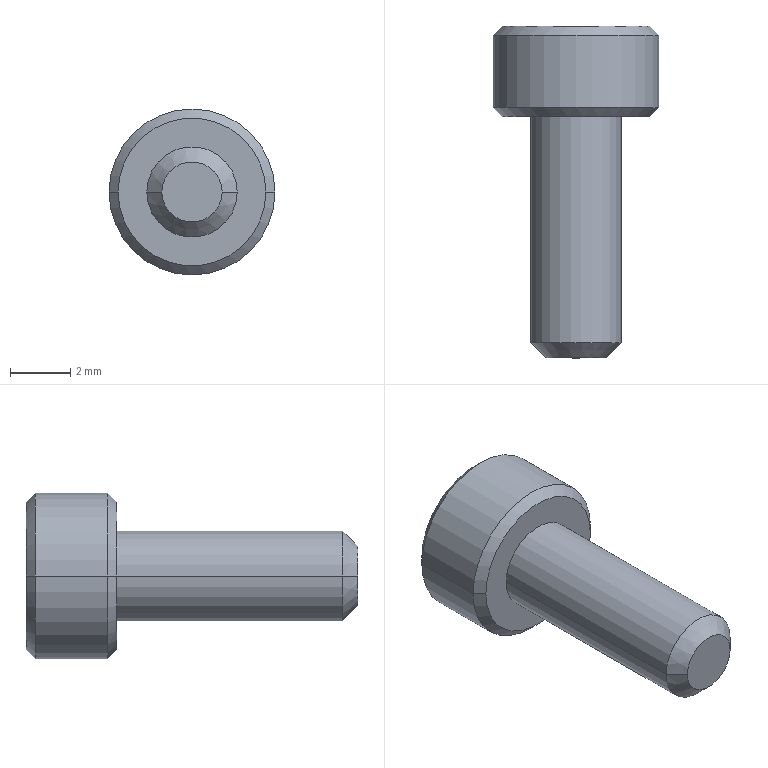Part | STEP file | BB62-M3-8L | 1 solid | 27 faces | box 5.5 x 11 x 5.5 mm | volume 116.536 mm3 | plane 15 | cone 8 | cylinder 4 | commonest cylinder face diameters 3 x2 5.5 x2
STEP:
#1=CARTESIAN_POINT('',(0.,0.8715,0.));
#2=VERTEX_POINT('',#1);
#3=CARTESIAN_POINT('',(1.435,1.7,0.));
#4=VERTEX_POINT('',#3);
#5=CARTESIAN_POINT('',(0.,0.8715,0.));
#6=DIRECTION('',(0.866,0.5,0.));
#7=VECTOR('',#6,1000.);
#8=LINE('',#5,#7);
#9=EDGE_CURVE('',#2,#4,#8,.T.);
#10=ORIENTED_EDGE('',*,*,#9,.F.);
#11=CARTESIAN_POINT('',(-1.435,1.7,0.));
#12=VERTEX_POINT('',#11);
#13=CARTESIAN_POINT('',(0.,0.8715,0.));
#14=DIRECTION('',(-0.866,0.5,0.));
#15=VECTOR('',#14,1000.);
#16=LINE('',#13,#15);
#17=EDGE_CURVE('',#2,#12,#16,.T.);
#18=ORIENTED_EDGE('',*,*,#17,.T.);
#19=CARTESIAN_POINT('',(-1.243,1.7,0.7175));
#20=VERTEX_POINT('',#19);
#21=CARTESIAN_POINT('',(0.,1.7,0.));
#22=DIRECTION('',(0.,-1.,0.));
#23=DIRECTION('',(-1.,0.,0.));
#24=AXIS2_PLACEMENT_3D('',#21,#22,#23);
#25=CIRCLE('',#24,1.435);
#26=EDGE_CURVE('',#20,#12,#25,.T.);
#27=ORIENTED_EDGE('',*,*,#26,.F.);
#28=CARTESIAN_POINT('',(0.,1.7,1.435));
#29=VERTEX_POINT('',#28);
#30=CARTESIAN_POINT('',(0.,1.7,0.));
#31=DIRECTION('',(0.,-1.,0.));
#32=DIRECTION('',(-1.,0.,0.));
#33=AXIS2_PLACEMENT_3D('',#30,#31,#32);
#34=CIRCLE('',#33,1.435);
#35=EDGE_CURVE('',#29,#20,#34,.T.);
#36=ORIENTED_EDGE('',*,*,#35,.F.);
#37=CARTESIAN_POINT('',(1.243,1.7,0.7175));
#38=VERTEX_POINT('',#37);
#39=CARTESIAN_POINT('',(0.,1.7,0.));
#40=DIRECTION('',(0.,-1.,0.));
#41=DIRECTION('',(-1.,0.,0.));
#42=AXIS2_PLACEMENT_3D('',#39,#40,#41);
#43=CIRCLE('',#42,1.435);
#44=EDGE_CURVE('',#38,#29,#43,.T.);
#45=ORIENTED_EDGE('',*,*,#44,.F.);
#46=CARTESIAN_POINT('',(0.,1.7,0.));
#47=DIRECTION('',(0.,-1.,0.));
#48=DIRECTION('',(-1.,0.,0.));
#49=AXIS2_PLACEMENT_3D('',#46,#47,#48);
#50=CIRCLE('',#49,1.435);
#51=EDGE_CURVE('',#4,#38,#50,.T.);
#52=ORIENTED_EDGE('',*,*,#51,.F.);
#53=EDGE_LOOP('',(#10,#18,#27,#36,#45,#52));
#54=FACE_OUTER_BOUND('',#53,.T.);
#55=CARTESIAN_POINT('',(0.,1000.872,0.));
#56=DIRECTION('',(0.,1.,0.));
#57=DIRECTION('',(1.,0.,0.));
#58=AXIS2_PLACEMENT_3D('',#55,#56,#57);
#59=CONICAL_SURFACE('',#58,1732.051,1.047);
#60=ADVANCED_FACE('',(#54),#59,.F.);
#61=CARTESIAN_POINT('',(1.,-8.,0.));
#62=VERTEX_POINT('',#61);
#63=CARTESIAN_POINT('',(-1.,-8.,0.));
#64=VERTEX_POINT('',#63);
#65=CARTESIAN_POINT('',(0.,-8.,0.));
#66=DIRECTION('',(0.,1.,0.));
#67=DIRECTION('',(1.,0.,0.));
#68=AXIS2_PLACEMENT_3D('',#65,#66,#67);
#69=CIRCLE('',#68,1.);
#70=EDGE_CURVE('',#62,#64,#69,.T.);
#71=ORIENTED_EDGE('',*,*,#70,.T.);
#72=CARTESIAN_POINT('',(-1.5,-7.5,0.));
#73=VERTEX_POINT('',#72);
#74=CARTESIAN_POINT('',(-1.,-8.,0.));
#75=DIRECTION('',(-0.7071,0.7071,0.));
#76=VECTOR('',#75,1000.);
#77=LINE('',#74,#76);
#78=EDGE_CURVE('',#64,#73,#77,.T.);
#79=ORIENTED_EDGE('',*,*,#78,.T.);
#80=CARTESIAN_POINT('',(1.5,-7.5,0.));
#81=VERTEX_POINT('',#80);
#82=CARTESIAN_POINT('',(0.,-7.5,0.));
#83=DIRECTION('',(0.,-1.,0.));
#84=DIRECTION('',(-1.,0.,0.));
#85=AXIS2_PLACEMENT_3D('',#82,#83,#84);
#86=CIRCLE('',#85,1.5);
#87=EDGE_CURVE('',#73,#81,#86,.T.);
#88=ORIENTED_EDGE('',*,*,#87,.T.);
#89=CARTESIAN_POINT('',(1.,-8.,0.));
#90=DIRECTION('',(0.7071,0.7071,0.));
#91=VECTOR('',#90,1000.);
#92=LINE('',#89,#91);
#93=EDGE_CURVE('',#62,#81,#92,.T.);
#94=ORIENTED_EDGE('',*,*,#93,.F.);
#95=EDGE_LOOP('',(#71,#79,#88,#94));
#96=FACE_OUTER_BOUND('',#95,.T.);
#97=CARTESIAN_POINT('',(0.,-8.,0.));
#98=DIRECTION('',(0.,1.,0.));
#99=DIRECTION('',(1.,0.,0.));
#100=AXIS2_PLACEMENT_3D('',#97,#98,#99);
#101=CONICAL_SURFACE('',#100,1.,0.7854);
#102=ADVANCED_FACE('',(#96),#101,.T.);
#103=ORIENTED_EDGE('',*,*,#87,.F.);
#104=CARTESIAN_POINT('',(-1.5,0.,0.));
#105=VERTEX_POINT('',#104);
#106=CARTESIAN_POINT('',(-1.5,-7.5,0.));
#107=DIRECTION('',(0.,1.,0.));
#108=VECTOR('',#107,1000.);
#109=LINE('',#106,#108);
#110=EDGE_CURVE('',#73,#105,#109,.T.);
#111=ORIENTED_EDGE('',*,*,#110,.T.);
#112=CARTESIAN_POINT('',(1.5,0.,0.));
#113=VERTEX_POINT('',#112);
#114=CARTESIAN_POINT('',(0.,0.,0.));
#115=DIRECTION('',(0.,-1.,0.));
#116=DIRECTION('',(-1.,0.,0.));
#117=AXIS2_PLACEMENT_3D('',#114,#115,#116);
#118=CIRCLE('',#117,1.5);
#119=EDGE_CURVE('',#105,#113,#118,.T.);
#120=ORIENTED_EDGE('',*,*,#119,.T.);
#121=CARTESIAN_POINT('',(1.5,-7.5,0.));
#122=DIRECTION('',(0.,1.,0.));
#123=VECTOR('',#122,1000.);
#124=LINE('',#121,#123);
#125=EDGE_CURVE('',#81,#113,#124,.T.);
#126=ORIENTED_EDGE('',*,*,#125,.F.);
#127=EDGE_LOOP('',(#103,#111,#120,#126));
#128=FACE_OUTER_BOUND('',#127,.T.);
#129=CARTESIAN_POINT('',(0.,-7.5,0.));
#130=DIRECTION('',(0.,1.,0.));
#131=DIRECTION('',(1.,0.,0.));
#132=AXIS2_PLACEMENT_3D('',#129,#130,#131);
#133=CYLINDRICAL_SURFACE('',#132,1.5);
#134=ADVANCED_FACE('',(#128),#133,.T.);
#135=CARTESIAN_POINT('',(-2.45,3.,0.));
#136=VERTEX_POINT('',#135);
#137=CARTESIAN_POINT('',(2.45,3.,0.));
#138=VERTEX_POINT('',#137);
#139=CARTESIAN_POINT('',(0.,3.,0.));
#140=DIRECTION('',(0.,-1.,0.));
#141=DIRECTION('',(-1.,0.,0.));
#142=AXIS2_PLACEMENT_3D('',#139,#140,#141);
#143=CIRCLE('',#142,2.45);
#144=EDGE_CURVE('',#136,#138,#143,.T.);
#145=ORIENTED_EDGE('',*,*,#144,.T.);
#146=CARTESIAN_POINT('',(2.75,2.7,0.));
#147=VERTEX_POINT('',#146);
#148=CARTESIAN_POINT('',(2.75,2.7,0.));
#149=DIRECTION('',(0.7071,-0.7071,0.));
#150=VECTOR('',#149,1000.);
#151=LINE('',#148,#150);
#152=EDGE_CURVE('',#138,#147,#151,.T.);
#153=ORIENTED_EDGE('',*,*,#152,.T.);
#154=CARTESIAN_POINT('',(-2.75,2.7,0.));
#155=VERTEX_POINT('',#154);
#156=CARTESIAN_POINT('',(0.,2.7,0.));
#157=DIRECTION('',(0.,-1.,0.));
#158=DIRECTION('',(-1.,0.,0.));
#159=AXIS2_PLACEMENT_3D('',#156,#157,#158);
#160=CIRCLE('',#159,2.75);
#161=EDGE_CURVE('',#155,#147,#160,.T.);
#162=ORIENTED_EDGE('',*,*,#161,.F.);
#163=CARTESIAN_POINT('',(-2.75,2.7,0.));
#164=DIRECTION('',(-0.7071,-0.7071,0.));
#165=VECTOR('',#164,1000.);
#166=LINE('',#163,#165);
#167=EDGE_CURVE('',#136,#155,#166,.T.);
#168=ORIENTED_EDGE('',*,*,#167,.F.);
#169=EDGE_LOOP('',(#145,#153,#162,#168));
#170=FACE_OUTER_BOUND('',#169,.T.);
#171=CARTESIAN_POINT('',(0.,2.7,0.));
#172=DIRECTION('',(0.,-1.,0.));
#173=DIRECTION('',(-1.,0.,0.));
#174=AXIS2_PLACEMENT_3D('',#171,#172,#173);
#175=CONICAL_SURFACE('',#174,2.75,0.7854);
#176=ADVANCED_FACE('',(#170),#175,.T.);
#177=ORIENTED_EDGE('',*,*,#161,.T.);
#178=CARTESIAN_POINT('',(2.75,0.3,0.));
#179=VERTEX_POINT('',#178);
#180=CARTESIAN_POINT('',(2.75,1.62,0.));
#181=DIRECTION('',(0.,-1.,0.));
#182=VECTOR('',#181,1000.);
#183=LINE('',#180,#182);
#184=EDGE_CURVE('',#147,#179,#183,.T.);
#185=ORIENTED_EDGE('',*,*,#184,.T.);
#186=CARTESIAN_POINT('',(-2.75,0.3,0.));
#187=VERTEX_POINT('',#186);
#188=CARTESIAN_POINT('',(0.,0.3,0.));
#189=DIRECTION('',(0.,-1.,0.));
#190=DIRECTION('',(-1.,0.,0.));
#191=AXIS2_PLACEMENT_3D('',#188,#189,#190);
#192=CIRCLE('',#191,2.75);
#193=EDGE_CURVE('',#187,#179,#192,.T.);
#194=ORIENTED_EDGE('',*,*,#193,.F.);
#195=CARTESIAN_POINT('',(-2.75,1.62,0.));
#196=DIRECTION('',(0.,-1.,0.));
#197=VECTOR('',#196,1000.);
#198=LINE('',#195,#197);
#199=EDGE_CURVE('',#155,#187,#198,.T.);
#200=ORIENTED_EDGE('',*,*,#199,.F.);
#201=EDGE_LOOP('',(#177,#185,#194,#200));
#202=FACE_OUTER_BOUND('',#201,.T.);
#203=CARTESIAN_POINT('',(0.,1.62,0.));
#204=DIRECTION('',(0.,-1.,0.));
#205=DIRECTION('',(-1.,0.,0.));
#206=AXIS2_PLACEMENT_3D('',#203,#204,#205);
#207=CYLINDRICAL_SURFACE('',#206,2.75);
#208=ADVANCED_FACE('',(#202),#207,.T.);
#209=CARTESIAN_POINT('',(-2.45,0.,0.));
#210=VERTEX_POINT('',#209);
#211=CARTESIAN_POINT('',(2.45,0.,0.));
#212=VERTEX_POINT('',#211);
#213=CARTESIAN_POINT('',(0.,0.,0.));
#214=DIRECTION('',(0.,-1.,0.));
#215=DIRECTION('',(-1.,0.,0.));
#216=AXIS2_PLACEMENT_3D('',#213,#214,#215);
#217=CIRCLE('',#216,2.45);
#218=EDGE_CURVE('',#210,#212,#217,.T.);
#219=ORIENTED_EDGE('',*,*,#218,.F.);
#220=CARTESIAN_POINT('',(-2.45,0.,0.));
#221=DIRECTION('',(-0.7071,0.7071,0.));
#222=VECTOR('',#221,1000.);
#223=LINE('',#220,#222);
#224=EDGE_CURVE('',#210,#187,#223,.T.);
#225=ORIENTED_EDGE('',*,*,#224,.T.);
#226=ORIENTED_EDGE('',*,*,#193,.T.);
#227=CARTESIAN_POINT('',(2.45,0.,0.));
#228=DIRECTION('',(0.7071,0.7071,0.));
#229=VECTOR('',#228,1000.);
#230=LINE('',#227,#229);
#231=EDGE_CURVE('',#212,#179,#230,.T.);
#232=ORIENTED_EDGE('',*,*,#231,.F.);
#233=EDGE_LOOP('',(#219,#225,#226,#232));
#234=FACE_OUTER_BOUND('',#233,.T.);
#235=CARTESIAN_POINT('',(0.,0.,0.));
#236=DIRECTION('',(0.,1.,0.));
#237=DIRECTION('',(1.,0.,0.));
#238=AXIS2_PLACEMENT_3D('',#235,#236,#237);
#239=CONICAL_SURFACE('',#238,2.45,0.7854);
#240=ADVANCED_FACE('',(#234),#239,.T.);
#241=ORIENTED_EDGE('',*,*,#144,.F.);
#242=CARTESIAN_POINT('',(0.,3.,0.));
#243=DIRECTION('',(0.,-1.,0.));
#244=DIRECTION('',(-1.,0.,0.));
#245=AXIS2_PLACEMENT_3D('',#242,#243,#244);
#246=CIRCLE('',#245,2.45);
#247=EDGE_CURVE('',#138,#136,#246,.T.);
#248=ORIENTED_EDGE('',*,*,#247,.F.);
#249=EDGE_LOOP('',(#241,#248));
#250=FACE_OUTER_BOUND('',#249,.T.);
#251=CARTESIAN_POINT('',(0.,3.,-1.435));
#252=VERTEX_POINT('',#251);
#253=CARTESIAN_POINT('',(-1.243,3.,-0.7175));
#254=VERTEX_POINT('',#253);
#255=CARTESIAN_POINT('',(0.,3.,-1.435));
#256=DIRECTION('',(-0.866,0.,0.5));
#257=VECTOR('',#256,1000.);
#258=LINE('',#255,#257);
#259=EDGE_CURVE('',#252,#254,#258,.T.);
#260=ORIENTED_EDGE('',*,*,#259,.F.);
#261=CARTESIAN_POINT('',(1.243,3.,-0.7175));
#262=VERTEX_POINT('',#261);
#263=CARTESIAN_POINT('',(1.243,3.,-0.7175));
#264=DIRECTION('',(-0.866,0.,-0.5));
#265=VECTOR('',#264,1000.);
#266=LINE('',#263,#265);
#267=EDGE_CURVE('',#262,#252,#266,.T.);
#268=ORIENTED_EDGE('',*,*,#267,.F.);
#269=CARTESIAN_POINT('',(1.243,3.,0.7175));
#270=VERTEX_POINT('',#269);
#271=CARTESIAN_POINT('',(1.243,3.,0.7175));
#272=DIRECTION('',(0.,0.,-1.));
#273=VECTOR('',#272,1000.);
#274=LINE('',#271,#273);
#275=EDGE_CURVE('',#270,#262,#274,.T.);
#276=ORIENTED_EDGE('',*,*,#275,.F.);
#277=CARTESIAN_POINT('',(0.,3.,1.435));
#278=VERTEX_POINT('',#277);
#279=CARTESIAN_POINT('',(0.,3.,1.435));
#280=DIRECTION('',(0.866,0.,-0.5));
#281=VECTOR('',#280,1000.);
#282=LINE('',#279,#281);
#283=EDGE_CURVE('',#278,#270,#282,.T.);
#284=ORIENTED_EDGE('',*,*,#283,.F.);
#285=CARTESIAN_POINT('',(-1.243,3.,0.7175));
#286=VERTEX_POINT('',#285);
#287=CARTESIAN_POINT('',(-1.243,3.,0.7175));
#288=DIRECTION('',(0.866,0.,0.5));
#289=VECTOR('',#288,1000.);
#290=LINE('',#287,#289);
#291=EDGE_CURVE('',#286,#278,#290,.T.);
#292=ORIENTED_EDGE('',*,*,#291,.F.);
#293=CARTESIAN_POINT('',(-1.243,3.,-0.7175));
#294=DIRECTION('',(0.,0.,1.));
#295=VECTOR('',#294,1000.);
#296=LINE('',#293,#295);
#297=EDGE_CURVE('',#254,#286,#296,.T.);
#298=ORIENTED_EDGE('',*,*,#297,.F.);
#299=EDGE_LOOP('',(#260,#268,#276,#284,#292,#298));
#300=FACE_BOUND('',#299,.T.);
#301=CARTESIAN_POINT('',(2.45,3.,0.));
#302=DIRECTION('',(0.,1.,0.));
#303=DIRECTION('',(1.,0.,0.));
#304=AXIS2_PLACEMENT_3D('',#301,#302,#303);
#305=PLANE('',#304);
#306=ADVANCED_FACE('',(#250,#300),#305,.T.);
#307=CARTESIAN_POINT('',(0.,0.,0.));
#308=DIRECTION('',(0.,-1.,0.));
#309=DIRECTION('',(-1.,0.,0.));
#310=AXIS2_PLACEMENT_3D('',#307,#308,#309);
#311=CIRCLE('',#310,1.5);
#312=EDGE_CURVE('',#113,#105,#311,.T.);
#313=ORIENTED_EDGE('',*,*,#312,.F.);
#314=ORIENTED_EDGE('',*,*,#119,.F.);
#315=EDGE_LOOP('',(#313,#314));
#316=FACE_BOUND('',#315,.T.);
#317=CARTESIAN_POINT('',(0.,0.,0.));
#318=DIRECTION('',(0.,-1.,0.));
#319=DIRECTION('',(-1.,0.,0.));
#320=AXIS2_PLACEMENT_3D('',#317,#318,#319);
#321=CIRCLE('',#320,2.45);
#322=EDGE_CURVE('',#212,#210,#321,.T.);
#323=ORIENTED_EDGE('',*,*,#322,.T.);
#324=ORIENTED_EDGE('',*,*,#218,.T.);
#325=EDGE_LOOP('',(#323,#324));
#326=FACE_OUTER_BOUND('',#325,.T.);
#327=CARTESIAN_POINT('',(0.,0.,0.));
#328=DIRECTION('',(0.,-1.,0.));
#329=DIRECTION('',(-1.,0.,0.));
#330=AXIS2_PLACEMENT_3D('',#327,#328,#329);
#331=PLANE('',#330);
#332=ADVANCED_FACE('',(#316,#326),#331,.T.);
#333=ORIENTED_EDGE('',*,*,#224,.F.);
#334=ORIENTED_EDGE('',*,*,#322,.F.);
#335=ORIENTED_EDGE('',*,*,#231,.T.);
#336=CARTESIAN_POINT('',(0.,0.3,0.));
#337=DIRECTION('',(0.,-1.,0.));
#338=DIRECTION('',(-1.,0.,0.));
#339=AXIS2_PLACEMENT_3D('',#336,#337,#338);
#340=CIRCLE('',#339,2.75);
#341=EDGE_CURVE('',#179,#187,#340,.T.);
#342=ORIENTED_EDGE('',*,*,#341,.T.);
#343=EDGE_LOOP('',(#333,#334,#335,#342));
#344=FACE_OUTER_BOUND('',#343,.T.);
#345=CARTESIAN_POINT('',(0.,0.,0.));
#346=DIRECTION('',(0.,1.,0.));
#347=DIRECTION('',(1.,0.,0.));
#348=AXIS2_PLACEMENT_3D('',#345,#346,#347);
#349=CONICAL_SURFACE('',#348,2.45,0.7854);
#350=ADVANCED_FACE('',(#344),#349,.T.);
#351=ORIENTED_EDGE('',*,*,#184,.F.);
#352=CARTESIAN_POINT('',(0.,2.7,0.));
#353=DIRECTION('',(0.,-1.,0.));
#354=DIRECTION('',(-1.,0.,0.));
#355=AXIS2_PLACEMENT_3D('',#352,#353,#354);
#356=CIRCLE('',#355,2.75);
#357=EDGE_CURVE('',#147,#155,#356,.T.);
#358=ORIENTED_EDGE('',*,*,#357,.T.);
#359=ORIENTED_EDGE('',*,*,#199,.T.);
#360=ORIENTED_EDGE('',*,*,#341,.F.);
#361=EDGE_LOOP('',(#351,#358,#359,#360));
#362=FACE_OUTER_BOUND('',#361,.T.);
#363=CARTESIAN_POINT('',(0.,1.62,0.));
#364=DIRECTION('',(0.,-1.,0.));
#365=DIRECTION('',(-1.,0.,0.));
#366=AXIS2_PLACEMENT_3D('',#363,#364,#365);
#367=CYLINDRICAL_SURFACE('',#366,2.75);
#368=ADVANCED_FACE('',(#362),#367,.T.);
#369=ORIENTED_EDGE('',*,*,#152,.F.);
#370=ORIENTED_EDGE('',*,*,#247,.T.);
#371=ORIENTED_EDGE('',*,*,#167,.T.);
#372=ORIENTED_EDGE('',*,*,#357,.F.);
#373=EDGE_LOOP('',(#369,#370,#371,#372));
#374=FACE_OUTER_BOUND('',#373,.T.);
#375=CARTESIAN_POINT('',(0.,2.7,0.));
#376=DIRECTION('',(0.,-1.,0.));
#377=DIRECTION('',(-1.,0.,0.));
#378=AXIS2_PLACEMENT_3D('',#375,#376,#377);
#379=CONICAL_SURFACE('',#378,2.75,0.7854);
#380=ADVANCED_FACE('',(#374),#379,.T.);
#381=ORIENTED_EDGE('',*,*,#110,.F.);
#382=CARTESIAN_POINT('',(0.,-7.5,0.));
#383=DIRECTION('',(0.,-1.,0.));
#384=DIRECTION('',(-1.,0.,0.));
#385=AXIS2_PLACEMENT_3D('',#382,#383,#384);
#386=CIRCLE('',#385,1.5);
#387=EDGE_CURVE('',#81,#73,#386,.T.);
#388=ORIENTED_EDGE('',*,*,#387,.F.);
#389=ORIENTED_EDGE('',*,*,#125,.T.);
#390=ORIENTED_EDGE('',*,*,#312,.T.);
#391=EDGE_LOOP('',(#381,#388,#389,#390));
#392=FACE_OUTER_BOUND('',#391,.T.);
#393=CARTESIAN_POINT('',(0.,-7.5,0.));
#394=DIRECTION('',(0.,1.,0.));
#395=DIRECTION('',(1.,0.,0.));
#396=AXIS2_PLACEMENT_3D('',#393,#394,#395);
#397=CYLINDRICAL_SURFACE('',#396,1.5);
#398=ADVANCED_FACE('',(#392),#397,.T.);
#399=ORIENTED_EDGE('',*,*,#70,.F.);
#400=CARTESIAN_POINT('',(0.,-8.,0.));
#401=DIRECTION('',(0.,1.,0.));
#402=DIRECTION('',(1.,0.,0.));
#403=AXIS2_PLACEMENT_3D('',#400,#401,#402);
#404=CIRCLE('',#403,1.);
#405=EDGE_CURVE('',#64,#62,#404,.T.);
#406=ORIENTED_EDGE('',*,*,#405,.F.);
#407=EDGE_LOOP('',(#399,#406));
#408=FACE_OUTER_BOUND('',#407,.T.);
#409=CARTESIAN_POINT('',(0.,-8.,0.));
#410=DIRECTION('',(0.,-1.,0.));
#411=DIRECTION('',(-1.,0.,0.));
#412=AXIS2_PLACEMENT_3D('',#409,#410,#411);
#413=PLANE('',#412);
#414=ADVANCED_FACE('',(#408),#413,.T.);
#415=ORIENTED_EDGE('',*,*,#78,.F.);
#416=ORIENTED_EDGE('',*,*,#405,.T.);
#417=ORIENTED_EDGE('',*,*,#93,.T.);
#418=ORIENTED_EDGE('',*,*,#387,.T.);
#419=EDGE_LOOP('',(#415,#416,#417,#418));
#420=FACE_OUTER_BOUND('',#419,.T.);
#421=CARTESIAN_POINT('',(0.,-8.,0.));
#422=DIRECTION('',(0.,1.,0.));
#423=DIRECTION('',(1.,0.,0.));
#424=AXIS2_PLACEMENT_3D('',#421,#422,#423);
#425=CONICAL_SURFACE('',#424,1.,0.7854);
#426=ADVANCED_FACE('',(#420),#425,.T.);
#427=CARTESIAN_POINT('',(1.243,1.7,-0.7175));
#428=VERTEX_POINT('',#427);
#429=CARTESIAN_POINT('',(0.,1.7,-1.435));
#430=VERTEX_POINT('',#429);
#431=CARTESIAN_POINT('',(1.243,1.7,-0.7175));
#432=DIRECTION('',(-0.866,0.,-0.5));
#433=VECTOR('',#432,1000.);
#434=LINE('',#431,#433);
#435=EDGE_CURVE('',#428,#430,#434,.T.);
#436=ORIENTED_EDGE('',*,*,#435,.F.);
#437=CARTESIAN_POINT('',(1.243,3.,-0.7175));
#438=DIRECTION('',(0.,-1.,0.));
#439=VECTOR('',#438,1000.);
#440=LINE('',#437,#439);
#441=EDGE_CURVE('',#262,#428,#440,.T.);
#442=ORIENTED_EDGE('',*,*,#441,.F.);
#443=ORIENTED_EDGE('',*,*,#267,.T.);
#444=CARTESIAN_POINT('',(0.,3.,-1.435));
#445=DIRECTION('',(0.,-1.,0.));
#446=VECTOR('',#445,1000.);
#447=LINE('',#444,#446);
#448=EDGE_CURVE('',#252,#430,#447,.T.);
#449=ORIENTED_EDGE('',*,*,#448,.T.);
#450=EDGE_LOOP('',(#436,#442,#443,#449));
#451=FACE_OUTER_BOUND('',#450,.T.);
#452=CARTESIAN_POINT('',(1.243,3.,-0.7175));
#453=DIRECTION('',(-0.5,0.,0.866));
#454=DIRECTION('',(0.866,0.,0.5));
#455=AXIS2_PLACEMENT_3D('',#452,#453,#454);
#456=PLANE('',#455);
#457=ADVANCED_FACE('',(#451),#456,.T.);
#458=CARTESIAN_POINT('',(-1.243,1.7,-0.7175));
#459=VERTEX_POINT('',#458);
#460=CARTESIAN_POINT('',(0.,1.7,-1.435));
#461=DIRECTION('',(-0.866,0.,0.5));
#462=VECTOR('',#461,1000.);
#463=LINE('',#460,#462);
#464=EDGE_CURVE('',#430,#459,#463,.T.);
#465=ORIENTED_EDGE('',*,*,#464,.F.);
#466=ORIENTED_EDGE('',*,*,#448,.F.);
#467=ORIENTED_EDGE('',*,*,#259,.T.);
#468=CARTESIAN_POINT('',(-1.243,3.,-0.7175));
#469=DIRECTION('',(0.,-1.,0.));
#470=VECTOR('',#469,1000.);
#471=LINE('',#468,#470);
#472=EDGE_CURVE('',#254,#459,#471,.T.);
#473=ORIENTED_EDGE('',*,*,#472,.T.);
#474=EDGE_LOOP('',(#465,#466,#467,#473));
#475=FACE_OUTER_BOUND('',#474,.T.);
#476=CARTESIAN_POINT('',(0.,3.,-1.435));
#477=DIRECTION('',(0.5,0.,0.866));
#478=DIRECTION('',(0.866,0.,-0.5));
#479=AXIS2_PLACEMENT_3D('',#476,#477,#478);
#480=PLANE('',#479);
#481=ADVANCED_FACE('',(#475),#480,.T.);
#482=CARTESIAN_POINT('',(-1.243,1.7,-0.7175));
#483=DIRECTION('',(0.,0.,1.));
#484=VECTOR('',#483,1000.);
#485=LINE('',#482,#484);
#486=EDGE_CURVE('',#459,#20,#485,.T.);
#487=ORIENTED_EDGE('',*,*,#486,.F.);
#488=ORIENTED_EDGE('',*,*,#472,.F.);
#489=ORIENTED_EDGE('',*,*,#297,.T.);
#490=CARTESIAN_POINT('',(-1.243,3.,0.7175));
#491=DIRECTION('',(0.,-1.,0.));
#492=VECTOR('',#491,1000.);
#493=LINE('',#490,#492);
#494=EDGE_CURVE('',#286,#20,#493,.T.);
#495=ORIENTED_EDGE('',*,*,#494,.T.);
#496=EDGE_LOOP('',(#487,#488,#489,#495));
#497=FACE_OUTER_BOUND('',#496,.T.);
#498=CARTESIAN_POINT('',(-1.243,3.,-0.7175));
#499=DIRECTION('',(1.,0.,0.));
#500=DIRECTION('',(0.,0.,-1.));
#501=AXIS2_PLACEMENT_3D('',#498,#499,#500);
#502=PLANE('',#501);
#503=ADVANCED_FACE('',(#497),#502,.T.);
#504=CARTESIAN_POINT('',(-1.243,1.7,0.7175));
#505=DIRECTION('',(0.866,0.,0.5));
#506=VECTOR('',#505,1000.);
#507=LINE('',#504,#506);
#508=EDGE_CURVE('',#20,#29,#507,.T.);
#509=ORIENTED_EDGE('',*,*,#508,.F.);
#510=ORIENTED_EDGE('',*,*,#494,.F.);
#511=ORIENTED_EDGE('',*,*,#291,.T.);
#512=CARTESIAN_POINT('',(0.,3.,1.435));
#513=DIRECTION('',(0.,-1.,0.));
#514=VECTOR('',#513,1000.);
#515=LINE('',#512,#514);
#516=EDGE_CURVE('',#278,#29,#515,.T.);
#517=ORIENTED_EDGE('',*,*,#516,.T.);
#518=EDGE_LOOP('',(#509,#510,#511,#517));
#519=FACE_OUTER_BOUND('',#518,.T.);
#520=CARTESIAN_POINT('',(-1.243,3.,0.7175));
#521=DIRECTION('',(0.5,0.,-0.866));
#522=DIRECTION('',(-0.866,0.,-0.5));
#523=AXIS2_PLACEMENT_3D('',#520,#521,#522);
#524=PLANE('',#523);
#525=ADVANCED_FACE('',(#519),#524,.T.);
#526=CARTESIAN_POINT('',(0.,1.7,1.435));
#527=DIRECTION('',(0.866,0.,-0.5));
#528=VECTOR('',#527,1000.);
#529=LINE('',#526,#528);
#530=EDGE_CURVE('',#29,#38,#529,.T.);
#531=ORIENTED_EDGE('',*,*,#530,.F.);
#532=ORIENTED_EDGE('',*,*,#516,.F.);
#533=ORIENTED_EDGE('',*,*,#283,.T.);
#534=CARTESIAN_POINT('',(1.243,3.,0.7175));
#535=DIRECTION('',(0.,-1.,0.));
#536=VECTOR('',#535,1000.);
#537=LINE('',#534,#536);
#538=EDGE_CURVE('',#270,#38,#537,.T.);
#539=ORIENTED_EDGE('',*,*,#538,.T.);
#540=EDGE_LOOP('',(#531,#532,#533,#539));
#541=FACE_OUTER_BOUND('',#540,.T.);
#542=CARTESIAN_POINT('',(0.,3.,1.435));
#543=DIRECTION('',(-0.5,0.,-0.866));
#544=DIRECTION('',(-0.866,0.,0.5));
#545=AXIS2_PLACEMENT_3D('',#542,#543,#544);
#546=PLANE('',#545);
#547=ADVANCED_FACE('',(#541),#546,.T.);
#548=CARTESIAN_POINT('',(1.243,1.7,0.7175));
#549=DIRECTION('',(0.,0.,-1.));
#550=VECTOR('',#549,1000.);
#551=LINE('',#548,#550);
#552=EDGE_CURVE('',#38,#428,#551,.T.);
#553=ORIENTED_EDGE('',*,*,#552,.F.);
#554=ORIENTED_EDGE('',*,*,#538,.F.);
#555=ORIENTED_EDGE('',*,*,#275,.T.);
#556=ORIENTED_EDGE('',*,*,#441,.T.);
#557=EDGE_LOOP('',(#553,#554,#555,#556));
#558=FACE_OUTER_BOUND('',#557,.T.);
#559=CARTESIAN_POINT('',(1.243,3.,0.7175));
#560=DIRECTION('',(-1.,0.,0.));
#561=DIRECTION('',(0.,0.,1.));
#562=AXIS2_PLACEMENT_3D('',#559,#560,#561);
#563=PLANE('',#562);
#564=ADVANCED_FACE('',(#558),#563,.T.);
#565=ORIENTED_EDGE('',*,*,#435,.T.);
#566=CARTESIAN_POINT('',(0.,1.7,0.));
#567=DIRECTION('',(0.,-1.,0.));
#568=DIRECTION('',(-1.,0.,0.));
#569=AXIS2_PLACEMENT_3D('',#566,#567,#568);
#570=CIRCLE('',#569,1.435);
#571=EDGE_CURVE('',#430,#428,#570,.T.);
#572=ORIENTED_EDGE('',*,*,#571,.T.);
#573=EDGE_LOOP('',(#565,#572));
#574=FACE_OUTER_BOUND('',#573,.T.);
#575=CARTESIAN_POINT('',(0.,1.7,0.));
#576=DIRECTION('',(0.,1.,0.));
#577=DIRECTION('',(1.,0.,0.));
#578=AXIS2_PLACEMENT_3D('',#575,#576,#577);
#579=PLANE('',#578);
#580=ADVANCED_FACE('',(#574),#579,.F.);
#581=ORIENTED_EDGE('',*,*,#552,.T.);
#582=CARTESIAN_POINT('',(0.,1.7,0.));
#583=DIRECTION('',(0.,-1.,0.));
#584=DIRECTION('',(-1.,0.,0.));
#585=AXIS2_PLACEMENT_3D('',#582,#583,#584);
#586=CIRCLE('',#585,1.435);
#587=EDGE_CURVE('',#428,#4,#586,.T.);
#588=ORIENTED_EDGE('',*,*,#587,.T.);
#589=ORIENTED_EDGE('',*,*,#51,.T.);
#590=EDGE_LOOP('',(#581,#588,#589));
#591=FACE_OUTER_BOUND('',#590,.T.);
#592=CARTESIAN_POINT('',(0.,1.7,0.));
#593=DIRECTION('',(0.,1.,0.));
#594=DIRECTION('',(1.,0.,0.));
#595=AXIS2_PLACEMENT_3D('',#592,#593,#594);
#596=PLANE('',#595);
#597=ADVANCED_FACE('',(#591),#596,.F.);
#598=ORIENTED_EDGE('',*,*,#530,.T.);
#599=ORIENTED_EDGE('',*,*,#44,.T.);
#600=EDGE_LOOP('',(#598,#599));
#601=FACE_OUTER_BOUND('',#600,.T.);
#602=CARTESIAN_POINT('',(0.,1.7,0.));
#603=DIRECTION('',(0.,1.,0.));
#604=DIRECTION('',(1.,0.,0.));
#605=AXIS2_PLACEMENT_3D('',#602,#603,#604);
#606=PLANE('',#605);
#607=ADVANCED_FACE('',(#601),#606,.F.);
#608=ORIENTED_EDGE('',*,*,#508,.T.);
#609=ORIENTED_EDGE('',*,*,#35,.T.);
#610=EDGE_LOOP('',(#608,#609));
#611=FACE_OUTER_BOUND('',#610,.T.);
#612=CARTESIAN_POINT('',(0.,1.7,0.));
#613=DIRECTION('',(0.,1.,0.));
#614=DIRECTION('',(1.,0.,0.));
#615=AXIS2_PLACEMENT_3D('',#612,#613,#614);
#616=PLANE('',#615);
#617=ADVANCED_FACE('',(#611),#616,.F.);
#618=ORIENTED_EDGE('',*,*,#486,.T.);
#619=ORIENTED_EDGE('',*,*,#26,.T.);
#620=CARTESIAN_POINT('',(0.,1.7,0.));
#621=DIRECTION('',(0.,-1.,0.));
#622=DIRECTION('',(-1.,0.,0.));
#623=AXIS2_PLACEMENT_3D('',#620,#621,#622);
#624=CIRCLE('',#623,1.435);
#625=EDGE_CURVE('',#12,#459,#624,.T.);
#626=ORIENTED_EDGE('',*,*,#625,.T.);
#627=EDGE_LOOP('',(#618,#619,#626));
#628=FACE_OUTER_BOUND('',#627,.T.);
#629=CARTESIAN_POINT('',(0.,1.7,0.));
#630=DIRECTION('',(0.,1.,0.));
#631=DIRECTION('',(1.,0.,0.));
#632=AXIS2_PLACEMENT_3D('',#629,#630,#631);
#633=PLANE('',#632);
#634=ADVANCED_FACE('',(#628),#633,.F.);
#635=ORIENTED_EDGE('',*,*,#464,.T.);
#636=CARTESIAN_POINT('',(0.,1.7,0.));
#637=DIRECTION('',(0.,-1.,0.));
#638=DIRECTION('',(-1.,0.,0.));
#639=AXIS2_PLACEMENT_3D('',#636,#637,#638);
#640=CIRCLE('',#639,1.435);
#641=EDGE_CURVE('',#459,#430,#640,.T.);
#642=ORIENTED_EDGE('',*,*,#641,.T.);
#643=EDGE_LOOP('',(#635,#642));
#644=FACE_OUTER_BOUND('',#643,.T.);
#645=CARTESIAN_POINT('',(0.,1.7,0.));
#646=DIRECTION('',(0.,1.,0.));
#647=DIRECTION('',(1.,0.,0.));
#648=AXIS2_PLACEMENT_3D('',#645,#646,#647);
#649=PLANE('',#648);
#650=ADVANCED_FACE('',(#644),#649,.F.);
#651=ORIENTED_EDGE('',*,*,#17,.F.);
#652=ORIENTED_EDGE('',*,*,#9,.T.);
#653=ORIENTED_EDGE('',*,*,#587,.F.);
#654=ORIENTED_EDGE('',*,*,#571,.F.);
#655=ORIENTED_EDGE('',*,*,#641,.F.);
#656=ORIENTED_EDGE('',*,*,#625,.F.);
#657=EDGE_LOOP('',(#651,#652,#653,#654,#655,#656));
#658=FACE_OUTER_BOUND('',#657,.T.);
#659=CARTESIAN_POINT('',(0.,1000.872,0.));
#660=DIRECTION('',(0.,1.,0.));
#661=DIRECTION('',(1.,0.,0.));
#662=AXIS2_PLACEMENT_3D('',#659,#660,#661);
#663=CONICAL_SURFACE('',#662,1732.051,1.047);
#664=ADVANCED_FACE('',(#658),#663,.F.);
#665=CLOSED_SHELL('',(#60,#102,#134,#176,#208,#240,#306,#332,#350,#368,#380,#398,#414,#426,#457,#481,#503,#525,#547,#564,#580,#597,#607,#617,#634,#650,#664));
#666=MANIFOLD_SOLID_BREP('',#665);
#667=CARTESIAN_POINT('',(0.,0.,0.));
#668=DIRECTION('',(0.,0.,1.));
#669=DIRECTION('',(1.,0.,0.));
#670=AXIS2_PLACEMENT_3D('',#667,#668,#669);
#671=(LENGTH_UNIT()NAMED_UNIT(*)SI_UNIT(.MILLI.,.METRE.));
#672=UNCERTAINTY_MEASURE_WITH_UNIT(LENGTH_MEASURE(0.00001),#671,'','');
#673=(NAMED_UNIT(*)PLANE_ANGLE_UNIT()SI_UNIT($,.RADIAN.));
#674=(NAMED_UNIT(*)SI_UNIT($,.STERADIAN.)SOLID_ANGLE_UNIT());
#675=(GEOMETRIC_REPRESENTATION_CONTEXT(3)GLOBAL_UNCERTAINTY_ASSIGNED_CONTEXT((#672))GLOBAL_UNIT_ASSIGNED_CONTEXT((#671,#673,#674))REPRESENTATION_CONTEXT('',''));
#676=ADVANCED_BREP_SHAPE_REPRESENTATION('',(#666,#670),#675);